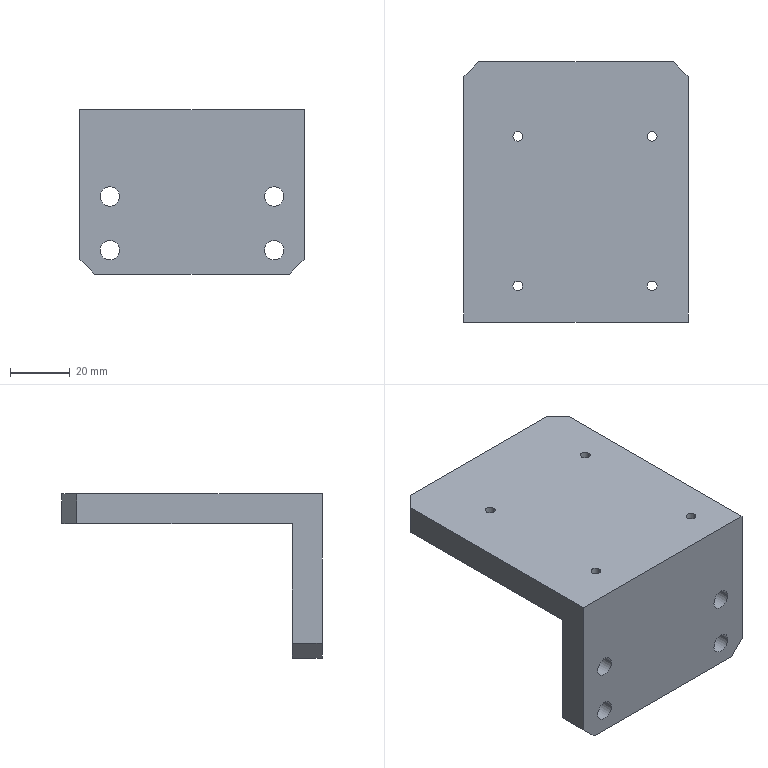Part | STEP file | ASND-0110-Body 1-25 | 1 solid | 28 faces | box 75 x 87.1 x 55 mm | volume 96917 mm3 | cylinder 16 | plane 12 | commonest cylinder face diameters 3.242 x8 6.5 x8